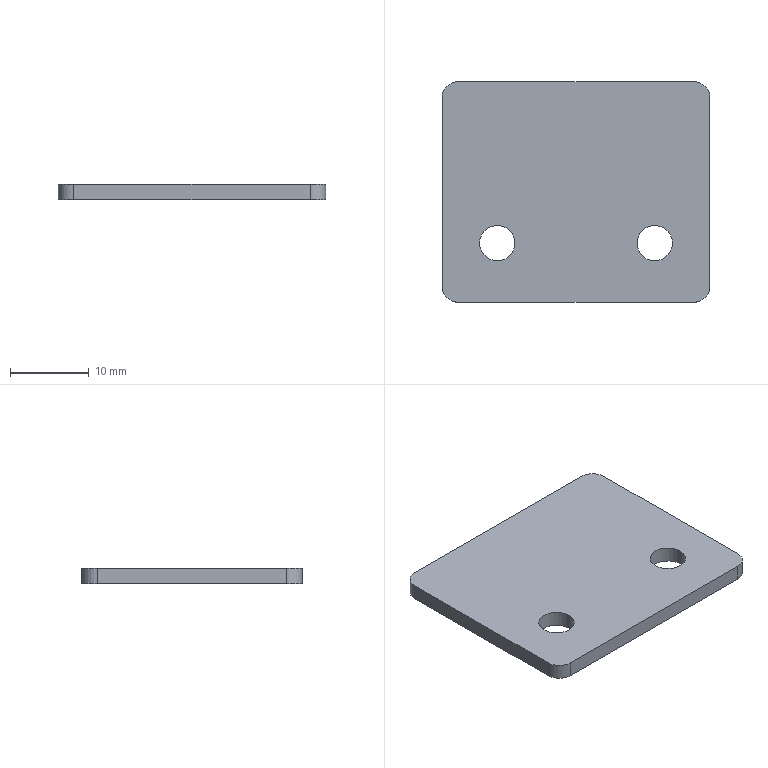Part | SolidWorks | features Extrusion 1, Fillet 1 | 1 solid | 14 faces | box 34 x 28 x 2 mm | volume 1834 mm3 | cylinder 8 | plane 6 | commonest cylinder face diameters 4 x4 4.5 x4
STEP:
#1=CARTESIAN_POINT('',(7.75,7.5,2.));
#2=VERTEX_POINT('',#1);
#3=CARTESIAN_POINT('',(12.25,7.5,2.));
#4=VERTEX_POINT('',#3);
#5=CARTESIAN_POINT('',(10.,7.5,2.));
#6=DIRECTION('',(0.,0.,1.));
#7=DIRECTION('',(-1.,0.,0.));
#8=AXIS2_PLACEMENT_3D('',#5,#6,#7);
#9=CIRCLE('',#8,2.25);
#10=EDGE_CURVE('',#2,#4,#9,.T.);
#11=ORIENTED_EDGE('',*,*,#10,.T.);
#12=CARTESIAN_POINT('',(12.25,7.5,0.));
#13=VERTEX_POINT('',#12);
#14=CARTESIAN_POINT('',(12.25,7.5,2.));
#15=DIRECTION('',(0.,0.,-1.));
#16=VECTOR('',#15,1000.);
#17=LINE('',#14,#16);
#18=EDGE_CURVE('',#4,#13,#17,.T.);
#19=ORIENTED_EDGE('',*,*,#18,.T.);
#20=CARTESIAN_POINT('',(7.75,7.5,0.));
#21=VERTEX_POINT('',#20);
#22=CARTESIAN_POINT('',(10.,7.5,0.));
#23=DIRECTION('',(0.,0.,1.));
#24=DIRECTION('',(-1.,0.,0.));
#25=AXIS2_PLACEMENT_3D('',#22,#23,#24);
#26=CIRCLE('',#25,2.25);
#27=EDGE_CURVE('',#21,#13,#26,.T.);
#28=ORIENTED_EDGE('',*,*,#27,.F.);
#29=CARTESIAN_POINT('',(7.75,7.5,2.));
#30=DIRECTION('',(0.,0.,-1.));
#31=VECTOR('',#30,1000.);
#32=LINE('',#29,#31);
#33=EDGE_CURVE('',#2,#21,#32,.T.);
#34=ORIENTED_EDGE('',*,*,#33,.F.);
#35=EDGE_LOOP('',(#11,#19,#28,#34));
#36=FACE_OUTER_BOUND('',#35,.T.);
#37=CARTESIAN_POINT('',(10.,7.5,2.));
#38=DIRECTION('',(0.,0.,-1.));
#39=DIRECTION('',(-1.,0.,0.));
#40=AXIS2_PLACEMENT_3D('',#37,#38,#39);
#41=CYLINDRICAL_SURFACE('',#40,2.25);
#42=ADVANCED_FACE('',(#36),#41,.F.);
#43=CARTESIAN_POINT('',(-12.25,7.5,2.));
#44=VERTEX_POINT('',#43);
#45=CARTESIAN_POINT('',(-7.75,7.5,2.));
#46=VERTEX_POINT('',#45);
#47=CARTESIAN_POINT('',(-10.,7.5,2.));
#48=DIRECTION('',(0.,0.,1.));
#49=DIRECTION('',(1.,0.,0.));
#50=AXIS2_PLACEMENT_3D('',#47,#48,#49);
#51=CIRCLE('',#50,2.25);
#52=EDGE_CURVE('',#44,#46,#51,.T.);
#53=ORIENTED_EDGE('',*,*,#52,.T.);
#54=CARTESIAN_POINT('',(-7.75,7.5,0.));
#55=VERTEX_POINT('',#54);
#56=CARTESIAN_POINT('',(-7.75,7.5,2.));
#57=DIRECTION('',(0.,0.,-1.));
#58=VECTOR('',#57,1000.);
#59=LINE('',#56,#58);
#60=EDGE_CURVE('',#46,#55,#59,.T.);
#61=ORIENTED_EDGE('',*,*,#60,.T.);
#62=CARTESIAN_POINT('',(-12.25,7.5,0.));
#63=VERTEX_POINT('',#62);
#64=CARTESIAN_POINT('',(-10.,7.5,0.));
#65=DIRECTION('',(0.,0.,1.));
#66=DIRECTION('',(1.,0.,0.));
#67=AXIS2_PLACEMENT_3D('',#64,#65,#66);
#68=CIRCLE('',#67,2.25);
#69=EDGE_CURVE('',#63,#55,#68,.T.);
#70=ORIENTED_EDGE('',*,*,#69,.F.);
#71=CARTESIAN_POINT('',(-12.25,7.5,2.));
#72=DIRECTION('',(0.,0.,-1.));
#73=VECTOR('',#72,1000.);
#74=LINE('',#71,#73);
#75=EDGE_CURVE('',#44,#63,#74,.T.);
#76=ORIENTED_EDGE('',*,*,#75,.F.);
#77=EDGE_LOOP('',(#53,#61,#70,#76));
#78=FACE_OUTER_BOUND('',#77,.T.);
#79=CARTESIAN_POINT('',(-10.,7.5,2.));
#80=DIRECTION('',(0.,0.,-1.));
#81=DIRECTION('',(-1.,0.,0.));
#82=AXIS2_PLACEMENT_3D('',#79,#80,#81);
#83=CYLINDRICAL_SURFACE('',#82,2.25);
#84=ADVANCED_FACE('',(#78),#83,.F.);
#85=ORIENTED_EDGE('',*,*,#52,.F.);
#86=CARTESIAN_POINT('',(-10.,7.5,2.));
#87=DIRECTION('',(0.,0.,1.));
#88=DIRECTION('',(1.,0.,0.));
#89=AXIS2_PLACEMENT_3D('',#86,#87,#88);
#90=CIRCLE('',#89,2.25);
#91=EDGE_CURVE('',#46,#44,#90,.T.);
#92=ORIENTED_EDGE('',*,*,#91,.F.);
#93=EDGE_LOOP('',(#85,#92));
#94=FACE_BOUND('',#93,.T.);
#95=CARTESIAN_POINT('',(15.,28.,2.));
#96=VERTEX_POINT('',#95);
#97=CARTESIAN_POINT('',(-15.,28.,2.));
#98=VERTEX_POINT('',#97);
#99=CARTESIAN_POINT('',(17.,28.,2.));
#100=DIRECTION('',(-1.,0.,0.));
#101=VECTOR('',#100,1000.);
#102=LINE('',#99,#101);
#103=EDGE_CURVE('',#96,#98,#102,.T.);
#104=ORIENTED_EDGE('',*,*,#103,.T.);
#105=CARTESIAN_POINT('',(-17.,26.,2.));
#106=VERTEX_POINT('',#105);
#107=CARTESIAN_POINT('',(-15.,26.,2.));
#108=DIRECTION('',(0.,0.,1.));
#109=DIRECTION('',(1.,0.,0.));
#110=AXIS2_PLACEMENT_3D('',#107,#108,#109);
#111=CIRCLE('',#110,2.);
#112=EDGE_CURVE('',#98,#106,#111,.T.);
#113=ORIENTED_EDGE('',*,*,#112,.T.);
#114=CARTESIAN_POINT('',(-17.,2.,2.));
#115=VERTEX_POINT('',#114);
#116=CARTESIAN_POINT('',(-17.,0.,2.));
#117=DIRECTION('',(0.,-1.,0.));
#118=VECTOR('',#117,1000.);
#119=LINE('',#116,#118);
#120=EDGE_CURVE('',#106,#115,#119,.T.);
#121=ORIENTED_EDGE('',*,*,#120,.T.);
#122=CARTESIAN_POINT('',(-15.,0.,2.));
#123=VERTEX_POINT('',#122);
#124=CARTESIAN_POINT('',(-15.,2.,2.));
#125=DIRECTION('',(0.,0.,1.));
#126=DIRECTION('',(1.,0.,0.));
#127=AXIS2_PLACEMENT_3D('',#124,#125,#126);
#128=CIRCLE('',#127,2.);
#129=EDGE_CURVE('',#115,#123,#128,.T.);
#130=ORIENTED_EDGE('',*,*,#129,.T.);
#131=CARTESIAN_POINT('',(15.,0.,2.));
#132=VERTEX_POINT('',#131);
#133=CARTESIAN_POINT('',(17.,0.,2.));
#134=DIRECTION('',(1.,0.,0.));
#135=VECTOR('',#134,1000.);
#136=LINE('',#133,#135);
#137=EDGE_CURVE('',#123,#132,#136,.T.);
#138=ORIENTED_EDGE('',*,*,#137,.T.);
#139=CARTESIAN_POINT('',(17.,2.,2.));
#140=VERTEX_POINT('',#139);
#141=CARTESIAN_POINT('',(15.,2.,2.));
#142=DIRECTION('',(0.,0.,1.));
#143=DIRECTION('',(1.,0.,0.));
#144=AXIS2_PLACEMENT_3D('',#141,#142,#143);
#145=CIRCLE('',#144,2.);
#146=EDGE_CURVE('',#132,#140,#145,.T.);
#147=ORIENTED_EDGE('',*,*,#146,.T.);
#148=CARTESIAN_POINT('',(17.,26.,2.));
#149=VERTEX_POINT('',#148);
#150=CARTESIAN_POINT('',(17.,0.,2.));
#151=DIRECTION('',(0.,1.,0.));
#152=VECTOR('',#151,1000.);
#153=LINE('',#150,#152);
#154=EDGE_CURVE('',#140,#149,#153,.T.);
#155=ORIENTED_EDGE('',*,*,#154,.T.);
#156=CARTESIAN_POINT('',(15.,26.,2.));
#157=DIRECTION('',(0.,0.,1.));
#158=DIRECTION('',(1.,0.,0.));
#159=AXIS2_PLACEMENT_3D('',#156,#157,#158);
#160=CIRCLE('',#159,2.);
#161=EDGE_CURVE('',#149,#96,#160,.T.);
#162=ORIENTED_EDGE('',*,*,#161,.T.);
#163=EDGE_LOOP('',(#104,#113,#121,#130,#138,#147,#155,#162));
#164=FACE_OUTER_BOUND('',#163,.T.);
#165=ORIENTED_EDGE('',*,*,#10,.F.);
#166=CARTESIAN_POINT('',(10.,7.5,2.));
#167=DIRECTION('',(0.,0.,1.));
#168=DIRECTION('',(-1.,0.,0.));
#169=AXIS2_PLACEMENT_3D('',#166,#167,#168);
#170=CIRCLE('',#169,2.25);
#171=EDGE_CURVE('',#4,#2,#170,.T.);
#172=ORIENTED_EDGE('',*,*,#171,.F.);
#173=EDGE_LOOP('',(#165,#172));
#174=FACE_BOUND('',#173,.T.);
#175=CARTESIAN_POINT('',(0.,0.,2.));
#176=DIRECTION('',(0.,0.,1.));
#177=DIRECTION('',(1.,0.,0.));
#178=AXIS2_PLACEMENT_3D('',#175,#176,#177);
#179=PLANE('',#178);
#180=ADVANCED_FACE('',(#94,#164,#174),#179,.T.);
#181=ORIENTED_EDGE('',*,*,#69,.T.);
#182=CARTESIAN_POINT('',(-10.,7.5,0.));
#183=DIRECTION('',(0.,0.,1.));
#184=DIRECTION('',(1.,0.,0.));
#185=AXIS2_PLACEMENT_3D('',#182,#183,#184);
#186=CIRCLE('',#185,2.25);
#187=EDGE_CURVE('',#55,#63,#186,.T.);
#188=ORIENTED_EDGE('',*,*,#187,.T.);
#189=EDGE_LOOP('',(#181,#188));
#190=FACE_BOUND('',#189,.T.);
#191=CARTESIAN_POINT('',(-17.,26.,0.));
#192=VERTEX_POINT('',#191);
#193=CARTESIAN_POINT('',(-17.,2.,0.));
#194=VERTEX_POINT('',#193);
#195=CARTESIAN_POINT('',(-17.,0.,0.));
#196=DIRECTION('',(0.,-1.,0.));
#197=VECTOR('',#196,1000.);
#198=LINE('',#195,#197);
#199=EDGE_CURVE('',#192,#194,#198,.T.);
#200=ORIENTED_EDGE('',*,*,#199,.F.);
#201=CARTESIAN_POINT('',(-15.,28.,0.));
#202=VERTEX_POINT('',#201);
#203=CARTESIAN_POINT('',(-15.,26.,0.));
#204=DIRECTION('',(0.,0.,-1.));
#205=DIRECTION('',(1.,0.,0.));
#206=AXIS2_PLACEMENT_3D('',#203,#204,#205);
#207=CIRCLE('',#206,2.);
#208=EDGE_CURVE('',#192,#202,#207,.T.);
#209=ORIENTED_EDGE('',*,*,#208,.T.);
#210=CARTESIAN_POINT('',(15.,28.,0.));
#211=VERTEX_POINT('',#210);
#212=CARTESIAN_POINT('',(17.,28.,0.));
#213=DIRECTION('',(-1.,0.,0.));
#214=VECTOR('',#213,1000.);
#215=LINE('',#212,#214);
#216=EDGE_CURVE('',#211,#202,#215,.T.);
#217=ORIENTED_EDGE('',*,*,#216,.F.);
#218=CARTESIAN_POINT('',(17.,26.,0.));
#219=VERTEX_POINT('',#218);
#220=CARTESIAN_POINT('',(15.,26.,0.));
#221=DIRECTION('',(0.,0.,-1.));
#222=DIRECTION('',(1.,0.,0.));
#223=AXIS2_PLACEMENT_3D('',#220,#221,#222);
#224=CIRCLE('',#223,2.);
#225=EDGE_CURVE('',#211,#219,#224,.T.);
#226=ORIENTED_EDGE('',*,*,#225,.T.);
#227=CARTESIAN_POINT('',(17.,2.,0.));
#228=VERTEX_POINT('',#227);
#229=CARTESIAN_POINT('',(17.,0.,0.));
#230=DIRECTION('',(0.,1.,0.));
#231=VECTOR('',#230,1000.);
#232=LINE('',#229,#231);
#233=EDGE_CURVE('',#228,#219,#232,.T.);
#234=ORIENTED_EDGE('',*,*,#233,.F.);
#235=CARTESIAN_POINT('',(15.,0.,0.));
#236=VERTEX_POINT('',#235);
#237=CARTESIAN_POINT('',(15.,2.,0.));
#238=DIRECTION('',(0.,0.,-1.));
#239=DIRECTION('',(1.,0.,0.));
#240=AXIS2_PLACEMENT_3D('',#237,#238,#239);
#241=CIRCLE('',#240,2.);
#242=EDGE_CURVE('',#228,#236,#241,.T.);
#243=ORIENTED_EDGE('',*,*,#242,.T.);
#244=CARTESIAN_POINT('',(-15.,0.,0.));
#245=VERTEX_POINT('',#244);
#246=CARTESIAN_POINT('',(17.,0.,0.));
#247=DIRECTION('',(1.,0.,0.));
#248=VECTOR('',#247,1000.);
#249=LINE('',#246,#248);
#250=EDGE_CURVE('',#245,#236,#249,.T.);
#251=ORIENTED_EDGE('',*,*,#250,.F.);
#252=CARTESIAN_POINT('',(-15.,2.,0.));
#253=DIRECTION('',(0.,0.,-1.));
#254=DIRECTION('',(1.,0.,0.));
#255=AXIS2_PLACEMENT_3D('',#252,#253,#254);
#256=CIRCLE('',#255,2.);
#257=EDGE_CURVE('',#245,#194,#256,.T.);
#258=ORIENTED_EDGE('',*,*,#257,.T.);
#259=EDGE_LOOP('',(#200,#209,#217,#226,#234,#243,#251,#258));
#260=FACE_OUTER_BOUND('',#259,.T.);
#261=ORIENTED_EDGE('',*,*,#27,.T.);
#262=CARTESIAN_POINT('',(10.,7.5,0.));
#263=DIRECTION('',(0.,0.,1.));
#264=DIRECTION('',(-1.,0.,0.));
#265=AXIS2_PLACEMENT_3D('',#262,#263,#264);
#266=CIRCLE('',#265,2.25);
#267=EDGE_CURVE('',#13,#21,#266,.T.);
#268=ORIENTED_EDGE('',*,*,#267,.T.);
#269=EDGE_LOOP('',(#261,#268));
#270=FACE_BOUND('',#269,.T.);
#271=CARTESIAN_POINT('',(0.,0.,0.));
#272=DIRECTION('',(0.,0.,1.));
#273=DIRECTION('',(1.,0.,0.));
#274=AXIS2_PLACEMENT_3D('',#271,#272,#273);
#275=PLANE('',#274);
#276=ADVANCED_FACE('',(#190,#260,#270),#275,.F.);
#277=ORIENTED_EDGE('',*,*,#233,.T.);
#278=CARTESIAN_POINT('',(17.,26.,2.));
#279=DIRECTION('',(0.,0.,1.));
#280=VECTOR('',#279,1000.);
#281=LINE('',#278,#280);
#282=EDGE_CURVE('',#219,#149,#281,.T.);
#283=ORIENTED_EDGE('',*,*,#282,.T.);
#284=ORIENTED_EDGE('',*,*,#154,.F.);
#285=CARTESIAN_POINT('',(17.,2.,2.));
#286=DIRECTION('',(0.,0.,-1.));
#287=VECTOR('',#286,1000.);
#288=LINE('',#285,#287);
#289=EDGE_CURVE('',#140,#228,#288,.T.);
#290=ORIENTED_EDGE('',*,*,#289,.T.);
#291=EDGE_LOOP('',(#277,#283,#284,#290));
#292=FACE_OUTER_BOUND('',#291,.T.);
#293=CARTESIAN_POINT('',(17.,0.,2.));
#294=DIRECTION('',(-1.,0.,0.));
#295=DIRECTION('',(0.,0.,1.));
#296=AXIS2_PLACEMENT_3D('',#293,#294,#295);
#297=PLANE('',#296);
#298=ADVANCED_FACE('',(#292),#297,.F.);
#299=ORIENTED_EDGE('',*,*,#216,.T.);
#300=CARTESIAN_POINT('',(-15.,28.,2.));
#301=DIRECTION('',(0.,0.,1.));
#302=VECTOR('',#301,1000.);
#303=LINE('',#300,#302);
#304=EDGE_CURVE('',#202,#98,#303,.T.);
#305=ORIENTED_EDGE('',*,*,#304,.T.);
#306=ORIENTED_EDGE('',*,*,#103,.F.);
#307=CARTESIAN_POINT('',(15.,28.,2.));
#308=DIRECTION('',(0.,0.,-1.));
#309=VECTOR('',#308,1000.);
#310=LINE('',#307,#309);
#311=EDGE_CURVE('',#96,#211,#310,.T.);
#312=ORIENTED_EDGE('',*,*,#311,.T.);
#313=EDGE_LOOP('',(#299,#305,#306,#312));
#314=FACE_OUTER_BOUND('',#313,.T.);
#315=CARTESIAN_POINT('',(17.,28.,2.));
#316=DIRECTION('',(0.,-1.,0.));
#317=DIRECTION('',(0.,0.,-1.));
#318=AXIS2_PLACEMENT_3D('',#315,#316,#317);
#319=PLANE('',#318);
#320=ADVANCED_FACE('',(#314),#319,.F.);
#321=ORIENTED_EDGE('',*,*,#120,.F.);
#322=CARTESIAN_POINT('',(-17.,26.,2.));
#323=DIRECTION('',(0.,0.,-1.));
#324=VECTOR('',#323,1000.);
#325=LINE('',#322,#324);
#326=EDGE_CURVE('',#106,#192,#325,.T.);
#327=ORIENTED_EDGE('',*,*,#326,.T.);
#328=ORIENTED_EDGE('',*,*,#199,.T.);
#329=CARTESIAN_POINT('',(-17.,2.,2.));
#330=DIRECTION('',(0.,0.,1.));
#331=VECTOR('',#330,1000.);
#332=LINE('',#329,#331);
#333=EDGE_CURVE('',#194,#115,#332,.T.);
#334=ORIENTED_EDGE('',*,*,#333,.T.);
#335=EDGE_LOOP('',(#321,#327,#328,#334));
#336=FACE_OUTER_BOUND('',#335,.T.);
#337=CARTESIAN_POINT('',(-17.,0.,2.));
#338=DIRECTION('',(1.,0.,0.));
#339=DIRECTION('',(0.,0.,-1.));
#340=AXIS2_PLACEMENT_3D('',#337,#338,#339);
#341=PLANE('',#340);
#342=ADVANCED_FACE('',(#336),#341,.F.);
#343=ORIENTED_EDGE('',*,*,#137,.F.);
#344=CARTESIAN_POINT('',(-15.,0.,2.));
#345=DIRECTION('',(0.,0.,-1.));
#346=VECTOR('',#345,1000.);
#347=LINE('',#344,#346);
#348=EDGE_CURVE('',#123,#245,#347,.T.);
#349=ORIENTED_EDGE('',*,*,#348,.T.);
#350=ORIENTED_EDGE('',*,*,#250,.T.);
#351=CARTESIAN_POINT('',(15.,0.,2.));
#352=DIRECTION('',(0.,0.,1.));
#353=VECTOR('',#352,1000.);
#354=LINE('',#351,#353);
#355=EDGE_CURVE('',#236,#132,#354,.T.);
#356=ORIENTED_EDGE('',*,*,#355,.T.);
#357=EDGE_LOOP('',(#343,#349,#350,#356));
#358=FACE_OUTER_BOUND('',#357,.T.);
#359=CARTESIAN_POINT('',(17.,0.,2.));
#360=DIRECTION('',(0.,1.,0.));
#361=DIRECTION('',(0.,0.,1.));
#362=AXIS2_PLACEMENT_3D('',#359,#360,#361);
#363=PLANE('',#362);
#364=ADVANCED_FACE('',(#358),#363,.F.);
#365=ORIENTED_EDGE('',*,*,#60,.F.);
#366=ORIENTED_EDGE('',*,*,#91,.T.);
#367=ORIENTED_EDGE('',*,*,#75,.T.);
#368=ORIENTED_EDGE('',*,*,#187,.F.);
#369=EDGE_LOOP('',(#365,#366,#367,#368));
#370=FACE_OUTER_BOUND('',#369,.T.);
#371=CARTESIAN_POINT('',(-10.,7.5,2.));
#372=DIRECTION('',(0.,0.,-1.));
#373=DIRECTION('',(-1.,0.,0.));
#374=AXIS2_PLACEMENT_3D('',#371,#372,#373);
#375=CYLINDRICAL_SURFACE('',#374,2.25);
#376=ADVANCED_FACE('',(#370),#375,.F.);
#377=ORIENTED_EDGE('',*,*,#18,.F.);
#378=ORIENTED_EDGE('',*,*,#171,.T.);
#379=ORIENTED_EDGE('',*,*,#33,.T.);
#380=ORIENTED_EDGE('',*,*,#267,.F.);
#381=EDGE_LOOP('',(#377,#378,#379,#380));
#382=FACE_OUTER_BOUND('',#381,.T.);
#383=CARTESIAN_POINT('',(10.,7.5,2.));
#384=DIRECTION('',(0.,0.,-1.));
#385=DIRECTION('',(-1.,0.,0.));
#386=AXIS2_PLACEMENT_3D('',#383,#384,#385);
#387=CYLINDRICAL_SURFACE('',#386,2.25);
#388=ADVANCED_FACE('',(#382),#387,.F.);
#389=ORIENTED_EDGE('',*,*,#112,.F.);
#390=ORIENTED_EDGE('',*,*,#304,.F.);
#391=ORIENTED_EDGE('',*,*,#208,.F.);
#392=ORIENTED_EDGE('',*,*,#326,.F.);
#393=EDGE_LOOP('',(#389,#390,#391,#392));
#394=FACE_OUTER_BOUND('',#393,.T.);
#395=CARTESIAN_POINT('',(-15.,26.,2.));
#396=DIRECTION('',(0.,0.,-1.));
#397=DIRECTION('',(-1.,0.,0.));
#398=AXIS2_PLACEMENT_3D('',#395,#396,#397);
#399=CYLINDRICAL_SURFACE('',#398,2.);
#400=ADVANCED_FACE('',(#394),#399,.T.);
#401=ORIENTED_EDGE('',*,*,#161,.F.);
#402=ORIENTED_EDGE('',*,*,#282,.F.);
#403=ORIENTED_EDGE('',*,*,#225,.F.);
#404=ORIENTED_EDGE('',*,*,#311,.F.);
#405=EDGE_LOOP('',(#401,#402,#403,#404));
#406=FACE_OUTER_BOUND('',#405,.T.);
#407=CARTESIAN_POINT('',(15.,26.,2.));
#408=DIRECTION('',(0.,0.,-1.));
#409=DIRECTION('',(-1.,0.,0.));
#410=AXIS2_PLACEMENT_3D('',#407,#408,#409);
#411=CYLINDRICAL_SURFACE('',#410,2.);
#412=ADVANCED_FACE('',(#406),#411,.T.);
#413=ORIENTED_EDGE('',*,*,#129,.F.);
#414=ORIENTED_EDGE('',*,*,#333,.F.);
#415=ORIENTED_EDGE('',*,*,#257,.F.);
#416=ORIENTED_EDGE('',*,*,#348,.F.);
#417=EDGE_LOOP('',(#413,#414,#415,#416));
#418=FACE_OUTER_BOUND('',#417,.T.);
#419=CARTESIAN_POINT('',(-15.,2.,2.));
#420=DIRECTION('',(0.,0.,-1.));
#421=DIRECTION('',(-1.,0.,0.));
#422=AXIS2_PLACEMENT_3D('',#419,#420,#421);
#423=CYLINDRICAL_SURFACE('',#422,2.);
#424=ADVANCED_FACE('',(#418),#423,.T.);
#425=ORIENTED_EDGE('',*,*,#146,.F.);
#426=ORIENTED_EDGE('',*,*,#355,.F.);
#427=ORIENTED_EDGE('',*,*,#242,.F.);
#428=ORIENTED_EDGE('',*,*,#289,.F.);
#429=EDGE_LOOP('',(#425,#426,#427,#428));
#430=FACE_OUTER_BOUND('',#429,.T.);
#431=CARTESIAN_POINT('',(15.,2.,2.));
#432=DIRECTION('',(0.,0.,-1.));
#433=DIRECTION('',(-1.,0.,0.));
#434=AXIS2_PLACEMENT_3D('',#431,#432,#433);
#435=CYLINDRICAL_SURFACE('',#434,2.);
#436=ADVANCED_FACE('',(#430),#435,.T.);
#437=CLOSED_SHELL('',(#42,#84,#180,#276,#298,#320,#342,#364,#376,#388,#400,#412,#424,#436));
#438=MANIFOLD_SOLID_BREP('',#437);
#439=CARTESIAN_POINT('',(0.,0.,0.));
#440=DIRECTION('',(0.,0.,1.));
#441=DIRECTION('',(1.,0.,0.));
#442=AXIS2_PLACEMENT_3D('',#439,#440,#441);
#443=(LENGTH_UNIT()NAMED_UNIT(*)SI_UNIT(.MILLI.,.METRE.));
#444=UNCERTAINTY_MEASURE_WITH_UNIT(LENGTH_MEASURE(0.00001),#443,'','');
#445=(NAMED_UNIT(*)PLANE_ANGLE_UNIT()SI_UNIT($,.RADIAN.));
#446=(NAMED_UNIT(*)SI_UNIT($,.STERADIAN.)SOLID_ANGLE_UNIT());
#447=(GEOMETRIC_REPRESENTATION_CONTEXT(3)GLOBAL_UNCERTAINTY_ASSIGNED_CONTEXT((#444))GLOBAL_UNIT_ASSIGNED_CONTEXT((#443,#445,#446))REPRESENTATION_CONTEXT('',''));
#448=ADVANCED_BREP_SHAPE_REPRESENTATION('',(#438,#442),#447);